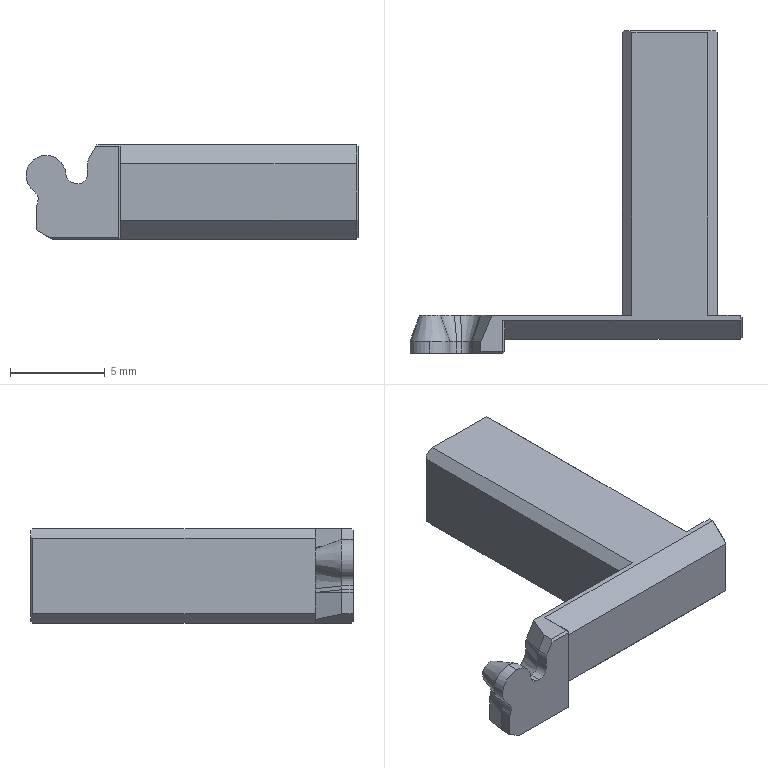Part | SolidWorks | features Chamfer 5, ICE 4, Cut 1, Extrusion 1, Fillet 1, HoleWzd 1 | 1 solid | 62 faces | box 17.497 x 17 x 5 mm | volume 457.03 mm3 | plane 45 | cylinder 9 | cone 8 | commonest cylinder face diameters 1 x5 1.6 x2 2.1 x2